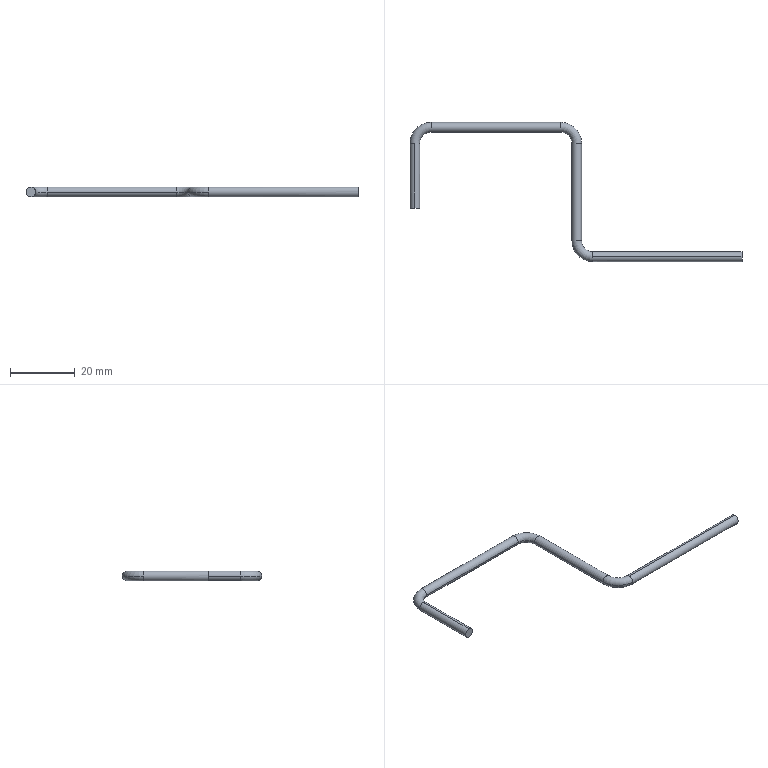Part | SolidWorks | features BaseBody 1 | 1 solid | 16 faces | box 102.526 x 43 x 3 mm | volume 1128 mm3 | cylinder 8 | torus 6 | plane 2 | commonest cylinder face diameters 3 x8
STEP:
#1=CARTESIAN_POINT('',(48.5,-10.,0.));
#2=VERTEX_POINT('',#1);
#3=CARTESIAN_POINT('',(51.5,-10.,0.));
#4=VERTEX_POINT('',#3);
#5=CARTESIAN_POINT('',(50.,-10.,0.));
#6=DIRECTION('',(0.,1.,0.));
#7=DIRECTION('',(0.,0.,1.));
#8=AXIS2_PLACEMENT_3D('',#5,#6,#7);
#9=CIRCLE('',#8,1.5);
#10=EDGE_CURVE('',#2,#4,#9,.T.);
#11=ORIENTED_EDGE('',*,*,#10,.F.);
#12=CARTESIAN_POINT('',(55.,-16.5,0.));
#13=VERTEX_POINT('',#12);
#14=CARTESIAN_POINT('',(55.,-10.,0.));
#15=DIRECTION('',(0.,0.,1.));
#16=DIRECTION('',(1.,0.,0.));
#17=AXIS2_PLACEMENT_3D('',#14,#15,#16);
#18=CIRCLE('',#17,6.5);
#19=EDGE_CURVE('',#2,#13,#18,.T.);
#20=ORIENTED_EDGE('',*,*,#19,.T.);
#21=CARTESIAN_POINT('',(55.,-15.,1.5));
#22=VERTEX_POINT('',#21);
#23=CARTESIAN_POINT('',(55.,-15.,0.));
#24=DIRECTION('',(-1.,0.,0.));
#25=DIRECTION('',(0.,0.,1.));
#26=AXIS2_PLACEMENT_3D('',#23,#24,#25);
#27=CIRCLE('',#26,1.5);
#28=EDGE_CURVE('',#13,#22,#27,.T.);
#29=ORIENTED_EDGE('',*,*,#28,.T.);
#30=CARTESIAN_POINT('',(55.,-13.5,0.));
#31=VERTEX_POINT('',#30);
#32=CARTESIAN_POINT('',(55.,-15.,0.));
#33=DIRECTION('',(-1.,0.,0.));
#34=DIRECTION('',(0.,0.,1.));
#35=AXIS2_PLACEMENT_3D('',#32,#33,#34);
#36=CIRCLE('',#35,1.5);
#37=EDGE_CURVE('',#22,#31,#36,.T.);
#38=ORIENTED_EDGE('',*,*,#37,.T.);
#39=CARTESIAN_POINT('',(55.,-10.,0.));
#40=DIRECTION('',(0.,0.,1.));
#41=DIRECTION('',(1.,0.,0.));
#42=AXIS2_PLACEMENT_3D('',#39,#40,#41);
#43=CIRCLE('',#42,3.5);
#44=EDGE_CURVE('',#4,#31,#43,.T.);
#45=ORIENTED_EDGE('',*,*,#44,.F.);
#46=EDGE_LOOP('',(#11,#20,#29,#38,#45));
#47=FACE_OUTER_BOUND('',#46,.T.);
#48=CARTESIAN_POINT('',(55.,-10.,0.));
#49=DIRECTION('',(0.,0.,1.));
#50=DIRECTION('',(1.,0.,0.));
#51=AXIS2_PLACEMENT_3D('',#48,#49,#50);
#52=TOROIDAL_SURFACE('',#51,5.,1.5);
#53=ADVANCED_FACE('',(#47),#52,.T.);
#54=CARTESIAN_POINT('',(45.,26.5,0.));
#55=VERTEX_POINT('',#54);
#56=CARTESIAN_POINT('',(45.,23.5,0.));
#57=VERTEX_POINT('',#56);
#58=CARTESIAN_POINT('',(45.,25.,0.));
#59=DIRECTION('',(-1.,0.,0.));
#60=DIRECTION('',(0.,0.,1.));
#61=AXIS2_PLACEMENT_3D('',#58,#59,#60);
#62=CIRCLE('',#61,1.5);
#63=EDGE_CURVE('',#55,#57,#62,.T.);
#64=ORIENTED_EDGE('',*,*,#63,.F.);
#65=CARTESIAN_POINT('',(51.5,20.,0.));
#66=VERTEX_POINT('',#65);
#67=CARTESIAN_POINT('',(45.,20.,0.));
#68=DIRECTION('',(0.,0.,-1.));
#69=DIRECTION('',(-1.,0.,0.));
#70=AXIS2_PLACEMENT_3D('',#67,#68,#69);
#71=CIRCLE('',#70,6.5);
#72=EDGE_CURVE('',#55,#66,#71,.T.);
#73=ORIENTED_EDGE('',*,*,#72,.T.);
#74=CARTESIAN_POINT('',(48.5,20.,0.));
#75=VERTEX_POINT('',#74);
#76=CARTESIAN_POINT('',(50.,20.,0.));
#77=DIRECTION('',(0.,1.,0.));
#78=DIRECTION('',(0.,0.,1.));
#79=AXIS2_PLACEMENT_3D('',#76,#77,#78);
#80=CIRCLE('',#79,1.5);
#81=EDGE_CURVE('',#66,#75,#80,.T.);
#82=ORIENTED_EDGE('',*,*,#81,.T.);
#83=CARTESIAN_POINT('',(45.,20.,0.));
#84=DIRECTION('',(0.,0.,-1.));
#85=DIRECTION('',(-1.,0.,0.));
#86=AXIS2_PLACEMENT_3D('',#83,#84,#85);
#87=CIRCLE('',#86,3.5);
#88=EDGE_CURVE('',#57,#75,#87,.T.);
#89=ORIENTED_EDGE('',*,*,#88,.F.);
#90=EDGE_LOOP('',(#64,#73,#82,#89));
#91=FACE_OUTER_BOUND('',#90,.T.);
#92=CARTESIAN_POINT('',(45.,20.,0.));
#93=DIRECTION('',(0.,0.,-1.));
#94=DIRECTION('',(-1.,0.,0.));
#95=AXIS2_PLACEMENT_3D('',#92,#93,#94);
#96=TOROIDAL_SURFACE('',#95,5.,1.5);
#97=ADVANCED_FACE('',(#91),#96,.T.);
#98=CARTESIAN_POINT('',(-1.5,20.,0.));
#99=VERTEX_POINT('',#98);
#100=CARTESIAN_POINT('',(0.,20.,-1.5));
#101=VERTEX_POINT('',#100);
#102=CARTESIAN_POINT('',(0.,20.,0.));
#103=DIRECTION('',(0.,-1.,0.));
#104=DIRECTION('',(0.,0.,1.));
#105=AXIS2_PLACEMENT_3D('',#102,#103,#104);
#106=CIRCLE('',#105,1.5);
#107=EDGE_CURVE('',#99,#101,#106,.T.);
#108=ORIENTED_EDGE('',*,*,#107,.F.);
#109=CARTESIAN_POINT('',(5.,26.5,0.));
#110=VERTEX_POINT('',#109);
#111=CARTESIAN_POINT('',(5.,20.,0.));
#112=DIRECTION('',(0.,0.,-1.));
#113=DIRECTION('',(-1.,0.,0.));
#114=AXIS2_PLACEMENT_3D('',#111,#112,#113);
#115=CIRCLE('',#114,6.5);
#116=EDGE_CURVE('',#99,#110,#115,.T.);
#117=ORIENTED_EDGE('',*,*,#116,.T.);
#118=CARTESIAN_POINT('',(5.,23.5,0.));
#119=VERTEX_POINT('',#118);
#120=CARTESIAN_POINT('',(5.,25.,0.));
#121=DIRECTION('',(-1.,0.,0.));
#122=DIRECTION('',(0.,0.,1.));
#123=AXIS2_PLACEMENT_3D('',#120,#121,#122);
#124=CIRCLE('',#123,1.5);
#125=EDGE_CURVE('',#110,#119,#124,.T.);
#126=ORIENTED_EDGE('',*,*,#125,.T.);
#127=CARTESIAN_POINT('',(1.5,20.,0.));
#128=VERTEX_POINT('',#127);
#129=CARTESIAN_POINT('',(5.,20.,0.));
#130=DIRECTION('',(0.,0.,-1.));
#131=DIRECTION('',(-1.,0.,0.));
#132=AXIS2_PLACEMENT_3D('',#129,#130,#131);
#133=CIRCLE('',#132,3.5);
#134=EDGE_CURVE('',#128,#119,#133,.T.);
#135=ORIENTED_EDGE('',*,*,#134,.F.);
#136=CARTESIAN_POINT('',(0.,20.,0.));
#137=DIRECTION('',(0.,-1.,0.));
#138=DIRECTION('',(0.,0.,1.));
#139=AXIS2_PLACEMENT_3D('',#136,#137,#138);
#140=CIRCLE('',#139,1.5);
#141=EDGE_CURVE('',#101,#128,#140,.T.);
#142=ORIENTED_EDGE('',*,*,#141,.F.);
#143=EDGE_LOOP('',(#108,#117,#126,#135,#142));
#144=FACE_OUTER_BOUND('',#143,.T.);
#145=CARTESIAN_POINT('',(5.,20.,0.));
#146=DIRECTION('',(0.,0.,-1.));
#147=DIRECTION('',(-1.,0.,0.));
#148=AXIS2_PLACEMENT_3D('',#145,#146,#147);
#149=TOROIDAL_SURFACE('',#148,5.,1.5);
#150=ADVANCED_FACE('',(#144),#149,.T.);
#151=ORIENTED_EDGE('',*,*,#37,.F.);
#152=CARTESIAN_POINT('',(101.026,-15.,1.5));
#153=VERTEX_POINT('',#152);
#154=CARTESIAN_POINT('',(55.,-15.,1.5));
#155=DIRECTION('',(1.,0.,0.));
#156=VECTOR('',#155,1000.);
#157=LINE('',#154,#156);
#158=EDGE_CURVE('',#22,#153,#157,.T.);
#159=ORIENTED_EDGE('',*,*,#158,.T.);
#160=CARTESIAN_POINT('',(101.026,-15.,-1.5));
#161=VERTEX_POINT('',#160);
#162=CARTESIAN_POINT('',(101.026,-15.,0.));
#163=DIRECTION('',(-1.,0.,0.));
#164=DIRECTION('',(0.,0.,1.));
#165=AXIS2_PLACEMENT_3D('',#162,#163,#164);
#166=CIRCLE('',#165,1.5);
#167=EDGE_CURVE('',#153,#161,#166,.T.);
#168=ORIENTED_EDGE('',*,*,#167,.T.);
#169=CARTESIAN_POINT('',(55.,-15.,-1.5));
#170=VERTEX_POINT('',#169);
#171=CARTESIAN_POINT('',(55.,-15.,-1.5));
#172=DIRECTION('',(1.,0.,0.));
#173=VECTOR('',#172,1000.);
#174=LINE('',#171,#173);
#175=EDGE_CURVE('',#170,#161,#174,.T.);
#176=ORIENTED_EDGE('',*,*,#175,.F.);
#177=CARTESIAN_POINT('',(55.,-15.,0.));
#178=DIRECTION('',(-1.,0.,0.));
#179=DIRECTION('',(0.,0.,1.));
#180=AXIS2_PLACEMENT_3D('',#177,#178,#179);
#181=CIRCLE('',#180,1.5);
#182=EDGE_CURVE('',#31,#170,#181,.T.);
#183=ORIENTED_EDGE('',*,*,#182,.F.);
#184=EDGE_LOOP('',(#151,#159,#168,#176,#183));
#185=FACE_OUTER_BOUND('',#184,.T.);
#186=CARTESIAN_POINT('',(55.,-15.,0.));
#187=DIRECTION('',(1.,0.,0.));
#188=DIRECTION('',(0.,0.,-1.));
#189=AXIS2_PLACEMENT_3D('',#186,#187,#188);
#190=CYLINDRICAL_SURFACE('',#189,1.5);
#191=ADVANCED_FACE('',(#185),#190,.T.);
#192=CARTESIAN_POINT('',(50.,20.,0.));
#193=DIRECTION('',(0.,1.,0.));
#194=DIRECTION('',(0.,0.,1.));
#195=AXIS2_PLACEMENT_3D('',#192,#193,#194);
#196=CIRCLE('',#195,1.5);
#197=EDGE_CURVE('',#75,#66,#196,.T.);
#198=ORIENTED_EDGE('',*,*,#197,.F.);
#199=CARTESIAN_POINT('',(48.5,20.,0.));
#200=DIRECTION('',(0.,-1.,0.));
#201=VECTOR('',#200,1000.);
#202=LINE('',#199,#201);
#203=EDGE_CURVE('',#75,#2,#202,.T.);
#204=ORIENTED_EDGE('',*,*,#203,.T.);
#205=ORIENTED_EDGE('',*,*,#10,.T.);
#206=CARTESIAN_POINT('',(51.5,20.,0.));
#207=DIRECTION('',(0.,-1.,0.));
#208=VECTOR('',#207,1000.);
#209=LINE('',#206,#208);
#210=EDGE_CURVE('',#66,#4,#209,.T.);
#211=ORIENTED_EDGE('',*,*,#210,.F.);
#212=EDGE_LOOP('',(#198,#204,#205,#211));
#213=FACE_OUTER_BOUND('',#212,.T.);
#214=CARTESIAN_POINT('',(50.,20.,0.));
#215=DIRECTION('',(0.,-1.,0.));
#216=DIRECTION('',(1.,0.,0.));
#217=AXIS2_PLACEMENT_3D('',#214,#215,#216);
#218=CYLINDRICAL_SURFACE('',#217,1.5);
#219=ADVANCED_FACE('',(#213),#218,.T.);
#220=CARTESIAN_POINT('',(5.,25.,0.));
#221=DIRECTION('',(-1.,0.,0.));
#222=DIRECTION('',(0.,0.,1.));
#223=AXIS2_PLACEMENT_3D('',#220,#221,#222);
#224=CIRCLE('',#223,1.5);
#225=EDGE_CURVE('',#119,#110,#224,.T.);
#226=ORIENTED_EDGE('',*,*,#225,.F.);
#227=CARTESIAN_POINT('',(5.,23.5,0.));
#228=DIRECTION('',(1.,0.,0.));
#229=VECTOR('',#228,1000.);
#230=LINE('',#227,#229);
#231=EDGE_CURVE('',#119,#57,#230,.T.);
#232=ORIENTED_EDGE('',*,*,#231,.T.);
#233=CARTESIAN_POINT('',(45.,25.,0.));
#234=DIRECTION('',(-1.,0.,0.));
#235=DIRECTION('',(0.,0.,1.));
#236=AXIS2_PLACEMENT_3D('',#233,#234,#235);
#237=CIRCLE('',#236,1.5);
#238=EDGE_CURVE('',#57,#55,#237,.T.);
#239=ORIENTED_EDGE('',*,*,#238,.T.);
#240=CARTESIAN_POINT('',(5.,26.5,0.));
#241=DIRECTION('',(1.,0.,0.));
#242=VECTOR('',#241,1000.);
#243=LINE('',#240,#242);
#244=EDGE_CURVE('',#110,#55,#243,.T.);
#245=ORIENTED_EDGE('',*,*,#244,.F.);
#246=EDGE_LOOP('',(#226,#232,#239,#245));
#247=FACE_OUTER_BOUND('',#246,.T.);
#248=CARTESIAN_POINT('',(5.,25.,0.));
#249=DIRECTION('',(1.,0.,0.));
#250=DIRECTION('',(0.,1.,0.));
#251=AXIS2_PLACEMENT_3D('',#248,#249,#250);
#252=CYLINDRICAL_SURFACE('',#251,1.5);
#253=ADVANCED_FACE('',(#247),#252,.T.);
#254=CARTESIAN_POINT('',(0.,0.,-1.5));
#255=VERTEX_POINT('',#254);
#256=CARTESIAN_POINT('',(0.,0.,1.5));
#257=VERTEX_POINT('',#256);
#258=CARTESIAN_POINT('',(0.,0.,0.));
#259=DIRECTION('',(0.,-1.,0.));
#260=DIRECTION('',(0.,0.,1.));
#261=AXIS2_PLACEMENT_3D('',#258,#259,#260);
#262=CIRCLE('',#261,1.5);
#263=EDGE_CURVE('',#255,#257,#262,.T.);
#264=ORIENTED_EDGE('',*,*,#263,.F.);
#265=CARTESIAN_POINT('',(0.,0.,-1.5));
#266=DIRECTION('',(0.,1.,0.));
#267=VECTOR('',#266,1000.);
#268=LINE('',#265,#267);
#269=EDGE_CURVE('',#255,#101,#268,.T.);
#270=ORIENTED_EDGE('',*,*,#269,.T.);
#271=ORIENTED_EDGE('',*,*,#141,.T.);
#272=CARTESIAN_POINT('',(0.,20.,1.5));
#273=VERTEX_POINT('',#272);
#274=CARTESIAN_POINT('',(0.,20.,0.));
#275=DIRECTION('',(0.,-1.,0.));
#276=DIRECTION('',(0.,0.,1.));
#277=AXIS2_PLACEMENT_3D('',#274,#275,#276);
#278=CIRCLE('',#277,1.5);
#279=EDGE_CURVE('',#128,#273,#278,.T.);
#280=ORIENTED_EDGE('',*,*,#279,.T.);
#281=CARTESIAN_POINT('',(0.,0.,1.5));
#282=DIRECTION('',(0.,1.,0.));
#283=VECTOR('',#282,1000.);
#284=LINE('',#281,#283);
#285=EDGE_CURVE('',#257,#273,#284,.T.);
#286=ORIENTED_EDGE('',*,*,#285,.F.);
#287=EDGE_LOOP('',(#264,#270,#271,#280,#286));
#288=FACE_OUTER_BOUND('',#287,.T.);
#289=CARTESIAN_POINT('',(0.,0.,0.));
#290=DIRECTION('',(0.,1.,0.));
#291=DIRECTION('',(0.,0.,1.));
#292=AXIS2_PLACEMENT_3D('',#289,#290,#291);
#293=CYLINDRICAL_SURFACE('',#292,1.5);
#294=ADVANCED_FACE('',(#288),#293,.T.);
#295=CARTESIAN_POINT('',(0.,0.,0.));
#296=DIRECTION('',(0.,-1.,0.));
#297=DIRECTION('',(0.,0.,1.));
#298=AXIS2_PLACEMENT_3D('',#295,#296,#297);
#299=CIRCLE('',#298,1.5);
#300=EDGE_CURVE('',#257,#255,#299,.T.);
#301=ORIENTED_EDGE('',*,*,#300,.T.);
#302=ORIENTED_EDGE('',*,*,#263,.T.);
#303=EDGE_LOOP('',(#301,#302));
#304=FACE_OUTER_BOUND('',#303,.T.);
#305=CARTESIAN_POINT('',(0.,0.,0.));
#306=DIRECTION('',(0.,-1.,0.));
#307=DIRECTION('',(0.,0.,1.));
#308=AXIS2_PLACEMENT_3D('',#305,#306,#307);
#309=PLANE('',#308);
#310=ADVANCED_FACE('',(#304),#309,.T.);
#311=CARTESIAN_POINT('',(101.026,-15.,0.));
#312=DIRECTION('',(-1.,0.,0.));
#313=DIRECTION('',(0.,0.,1.));
#314=AXIS2_PLACEMENT_3D('',#311,#312,#313);
#315=CIRCLE('',#314,1.5);
#316=EDGE_CURVE('',#161,#153,#315,.T.);
#317=ORIENTED_EDGE('',*,*,#316,.F.);
#318=ORIENTED_EDGE('',*,*,#167,.F.);
#319=EDGE_LOOP('',(#317,#318));
#320=FACE_OUTER_BOUND('',#319,.T.);
#321=CARTESIAN_POINT('',(101.026,-15.,0.));
#322=DIRECTION('',(-1.,0.,0.));
#323=DIRECTION('',(0.,0.,1.));
#324=AXIS2_PLACEMENT_3D('',#321,#322,#323);
#325=PLANE('',#324);
#326=ADVANCED_FACE('',(#320),#325,.F.);
#327=ORIENTED_EDGE('',*,*,#269,.F.);
#328=ORIENTED_EDGE('',*,*,#300,.F.);
#329=ORIENTED_EDGE('',*,*,#285,.T.);
#330=CARTESIAN_POINT('',(0.,20.,0.));
#331=DIRECTION('',(0.,-1.,0.));
#332=DIRECTION('',(0.,0.,1.));
#333=AXIS2_PLACEMENT_3D('',#330,#331,#332);
#334=CIRCLE('',#333,1.5);
#335=EDGE_CURVE('',#273,#99,#334,.T.);
#336=ORIENTED_EDGE('',*,*,#335,.T.);
#337=ORIENTED_EDGE('',*,*,#107,.T.);
#338=EDGE_LOOP('',(#327,#328,#329,#336,#337));
#339=FACE_OUTER_BOUND('',#338,.T.);
#340=CARTESIAN_POINT('',(0.,0.,0.));
#341=DIRECTION('',(0.,1.,0.));
#342=DIRECTION('',(0.,0.,1.));
#343=AXIS2_PLACEMENT_3D('',#340,#341,#342);
#344=CYLINDRICAL_SURFACE('',#343,1.5);
#345=ADVANCED_FACE('',(#339),#344,.T.);
#346=ORIENTED_EDGE('',*,*,#116,.F.);
#347=ORIENTED_EDGE('',*,*,#335,.F.);
#348=ORIENTED_EDGE('',*,*,#279,.F.);
#349=ORIENTED_EDGE('',*,*,#134,.T.);
#350=ORIENTED_EDGE('',*,*,#225,.T.);
#351=EDGE_LOOP('',(#346,#347,#348,#349,#350));
#352=FACE_OUTER_BOUND('',#351,.T.);
#353=CARTESIAN_POINT('',(5.,20.,0.));
#354=DIRECTION('',(0.,0.,-1.));
#355=DIRECTION('',(-1.,0.,0.));
#356=AXIS2_PLACEMENT_3D('',#353,#354,#355);
#357=TOROIDAL_SURFACE('',#356,5.,1.5);
#358=ADVANCED_FACE('',(#352),#357,.T.);
#359=ORIENTED_EDGE('',*,*,#231,.F.);
#360=ORIENTED_EDGE('',*,*,#125,.F.);
#361=ORIENTED_EDGE('',*,*,#244,.T.);
#362=ORIENTED_EDGE('',*,*,#63,.T.);
#363=EDGE_LOOP('',(#359,#360,#361,#362));
#364=FACE_OUTER_BOUND('',#363,.T.);
#365=CARTESIAN_POINT('',(5.,25.,0.));
#366=DIRECTION('',(1.,0.,0.));
#367=DIRECTION('',(0.,1.,0.));
#368=AXIS2_PLACEMENT_3D('',#365,#366,#367);
#369=CYLINDRICAL_SURFACE('',#368,1.5);
#370=ADVANCED_FACE('',(#364),#369,.T.);
#371=ORIENTED_EDGE('',*,*,#72,.F.);
#372=ORIENTED_EDGE('',*,*,#238,.F.);
#373=ORIENTED_EDGE('',*,*,#88,.T.);
#374=ORIENTED_EDGE('',*,*,#197,.T.);
#375=EDGE_LOOP('',(#371,#372,#373,#374));
#376=FACE_OUTER_BOUND('',#375,.T.);
#377=CARTESIAN_POINT('',(45.,20.,0.));
#378=DIRECTION('',(0.,0.,-1.));
#379=DIRECTION('',(-1.,0.,0.));
#380=AXIS2_PLACEMENT_3D('',#377,#378,#379);
#381=TOROIDAL_SURFACE('',#380,5.,1.5);
#382=ADVANCED_FACE('',(#376),#381,.T.);
#383=ORIENTED_EDGE('',*,*,#203,.F.);
#384=ORIENTED_EDGE('',*,*,#81,.F.);
#385=ORIENTED_EDGE('',*,*,#210,.T.);
#386=CARTESIAN_POINT('',(50.,-10.,0.));
#387=DIRECTION('',(0.,1.,0.));
#388=DIRECTION('',(0.,0.,1.));
#389=AXIS2_PLACEMENT_3D('',#386,#387,#388);
#390=CIRCLE('',#389,1.5);
#391=EDGE_CURVE('',#4,#2,#390,.T.);
#392=ORIENTED_EDGE('',*,*,#391,.T.);
#393=EDGE_LOOP('',(#383,#384,#385,#392));
#394=FACE_OUTER_BOUND('',#393,.T.);
#395=CARTESIAN_POINT('',(50.,20.,0.));
#396=DIRECTION('',(0.,-1.,0.));
#397=DIRECTION('',(1.,0.,0.));
#398=AXIS2_PLACEMENT_3D('',#395,#396,#397);
#399=CYLINDRICAL_SURFACE('',#398,1.5);
#400=ADVANCED_FACE('',(#394),#399,.T.);
#401=ORIENTED_EDGE('',*,*,#19,.F.);
#402=ORIENTED_EDGE('',*,*,#391,.F.);
#403=ORIENTED_EDGE('',*,*,#44,.T.);
#404=ORIENTED_EDGE('',*,*,#182,.T.);
#405=CARTESIAN_POINT('',(55.,-15.,0.));
#406=DIRECTION('',(-1.,0.,0.));
#407=DIRECTION('',(0.,0.,1.));
#408=AXIS2_PLACEMENT_3D('',#405,#406,#407);
#409=CIRCLE('',#408,1.5);
#410=EDGE_CURVE('',#170,#13,#409,.T.);
#411=ORIENTED_EDGE('',*,*,#410,.T.);
#412=EDGE_LOOP('',(#401,#402,#403,#404,#411));
#413=FACE_OUTER_BOUND('',#412,.T.);
#414=CARTESIAN_POINT('',(55.,-10.,0.));
#415=DIRECTION('',(0.,0.,1.));
#416=DIRECTION('',(1.,0.,0.));
#417=AXIS2_PLACEMENT_3D('',#414,#415,#416);
#418=TOROIDAL_SURFACE('',#417,5.,1.5);
#419=ADVANCED_FACE('',(#413),#418,.T.);
#420=ORIENTED_EDGE('',*,*,#158,.F.);
#421=ORIENTED_EDGE('',*,*,#28,.F.);
#422=ORIENTED_EDGE('',*,*,#410,.F.);
#423=ORIENTED_EDGE('',*,*,#175,.T.);
#424=ORIENTED_EDGE('',*,*,#316,.T.);
#425=EDGE_LOOP('',(#420,#421,#422,#423,#424));
#426=FACE_OUTER_BOUND('',#425,.T.);
#427=CARTESIAN_POINT('',(55.,-15.,0.));
#428=DIRECTION('',(1.,0.,0.));
#429=DIRECTION('',(0.,0.,-1.));
#430=AXIS2_PLACEMENT_3D('',#427,#428,#429);
#431=CYLINDRICAL_SURFACE('',#430,1.5);
#432=ADVANCED_FACE('',(#426),#431,.T.);
#433=CLOSED_SHELL('',(#53,#97,#150,#191,#219,#253,#294,#310,#326,#345,#358,#370,#382,#400,#419,#432));
#434=MANIFOLD_SOLID_BREP('',#433);
#435=CARTESIAN_POINT('',(0.,0.,0.));
#436=DIRECTION('',(0.,0.,1.));
#437=DIRECTION('',(1.,0.,0.));
#438=AXIS2_PLACEMENT_3D('',#435,#436,#437);
#439=(LENGTH_UNIT()NAMED_UNIT(*)SI_UNIT(.MILLI.,.METRE.));
#440=UNCERTAINTY_MEASURE_WITH_UNIT(LENGTH_MEASURE(0.00001),#439,'','');
#441=(NAMED_UNIT(*)PLANE_ANGLE_UNIT()SI_UNIT($,.RADIAN.));
#442=(NAMED_UNIT(*)SI_UNIT($,.STERADIAN.)SOLID_ANGLE_UNIT());
#443=(GEOMETRIC_REPRESENTATION_CONTEXT(3)GLOBAL_UNCERTAINTY_ASSIGNED_CONTEXT((#440))GLOBAL_UNIT_ASSIGNED_CONTEXT((#439,#441,#442))REPRESENTATION_CONTEXT('',''));
#444=ADVANCED_BREP_SHAPE_REPRESENTATION('',(#434,#438),#443);